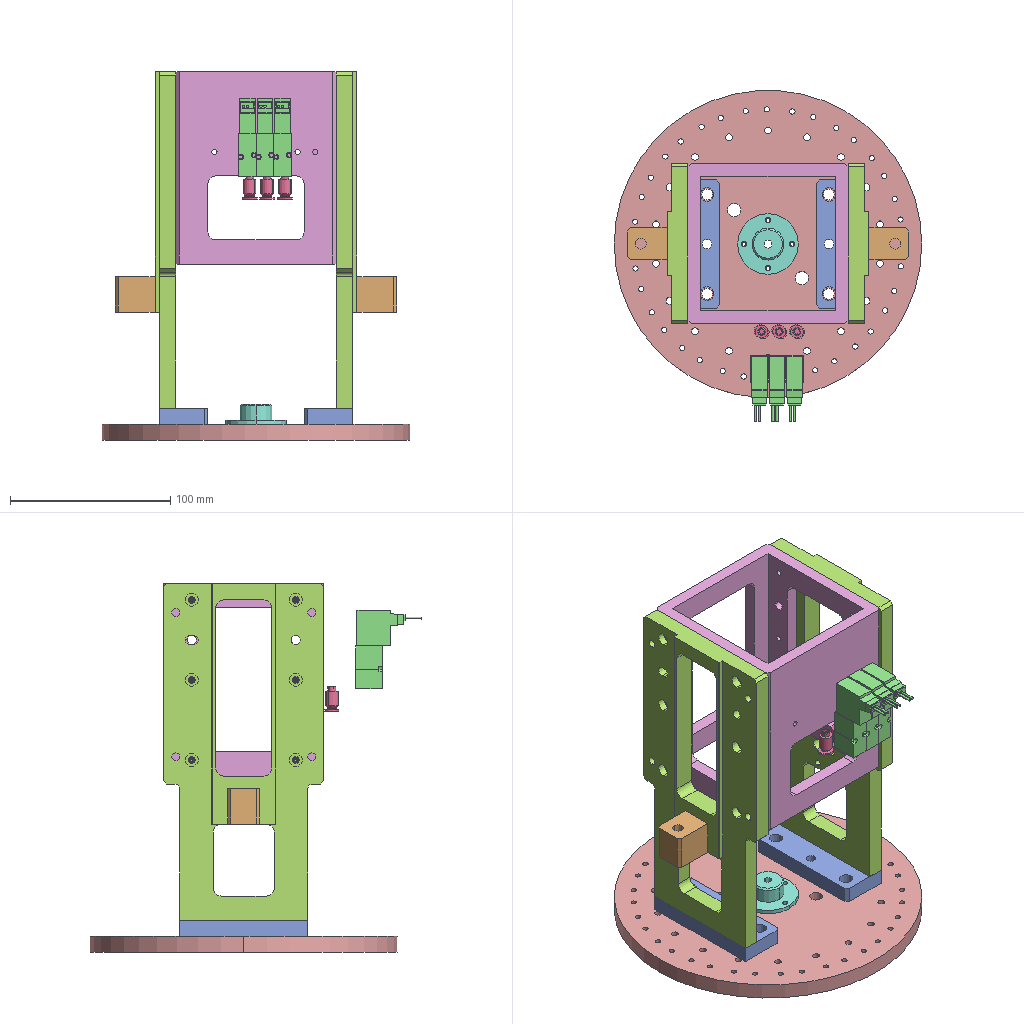Assembly | SolidWorks | 10 different items | 29 placed | box 192 x 207 x 230 mm
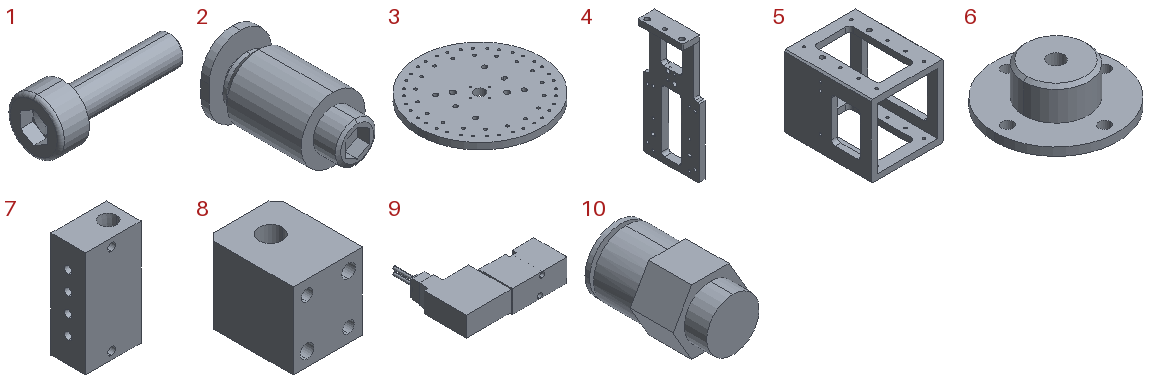Parts list (item | quantity | size | volume | features):
1 | x12 | 7.6 x 3 x 3 mm | 21.652 mm3 | features Fillet 2, RevCut 2, Boss 1, Chamfer 1, Cut 1, Extrusion 1, LPattern 1
2 | x4 | 8 x 15.6 x 9.8 mm | 520.13 mm3 | features BaseBody 1
3 | x1 | 192 x 192 x 10 mm | 278427 mm3 | features ICE 5, HoleWzd 3, 3DProfileFeature 2, CirPattern 2, Cut 2, Extrusion 1
4 | x2 | 33 x 100 x 220 mm | 162371 mm3 | features ICE 12, Chamfer 3, HoleWzd 3, Cut 2, Fillet 2, 3DProfileFeature 1, Extrusion 1
5 | x1 | 100 x 120 x 100 mm | 216402 mm3 | features ICE 5, HoleWzd 4, MirrorPattern 2, 3DProfileFeature 1, Chamfer 1, Cut 1, Extrusion 1
6 | x1 | 38 x 38 x 12.5 mm | 5119 mm3 | features ICE 2, Chamfer 1, Extrusion 1, HoleWzd 1
7 | x1 | 32 x 20 x 61 mm | 34864 mm3 | features HoleWzd 6, ICE 5, Extrusion 1, LPattern 1, RefAxis 1, RevCut 1
8 | x2 | 20 x 25 x 22 mm | 9700 mm3 | features HoleWzd 3, Chamfer 1, Extrusion 1
9 | x4 | 49 x 41 x 11 mm | 9805 mm3 | features BaseBody 1, ICE 1
10 | x1 | 13.856 x 21.6 x 12 mm | 1847 mm3 | features BaseBody 1
Mates (type | each side: item.copy, entity, surface, feature):
Coincident | 3.1 face plane Boss-Extrude1 | 4.1 face plane Boss-Extrude1
Coincident | 4.1 face plane Boss-Extrude1 | 5.1 face plane Boss-Extrude1
Coincident | 4.2 face plane Boss-Extrude1 | 5.1 face plane Boss-Extrude1
Concentric | 4.2 face cylinder Cut-Extrude7 | 5.1 face cylinder Mirror2
Concentric | 4.2 face cylinder Cut-Extrude8 | 5.1 face cylinder Mirror2
Concentric | 4.1 face cylinder Cut-Extrude7 | 1.1 face cylinder BaseBody
Coincident | 4.1 face plane Cut-Extrude8 | 1.1 face plane BaseHead
Concentric | 4.1 face cylinder Cut-Extrude7 | 1.2 face cylinder BaseBody
Coincident | 4.1 face plane Cut-Extrude8 | 1.2 face plane BaseHead
Concentric | 4.1 face cylinder Cut-Extrude7 | 1.3 face cylinder BaseBody
Coincident | 4.1 face plane Cut-Extrude8 | 1.3 face plane BaseHead
Concentric | 4.1 face cylinder Cut-Extrude7 | 1.4 face cylinder BaseBody
Coincident | 4.1 face plane Cut-Extrude8 | 1.4 face plane BaseHead
Concentric | 4.1 face cylinder Cut-Extrude7 | 1.5 face cylinder BaseBody
Coincident | 4.1 face plane Cut-Extrude8 | 1.5 face plane BaseHead
Concentric | 4.1 face cylinder Cut-Extrude7 | 1.6 face cylinder BaseBody
Coincident | 4.1 face plane Cut-Extrude8 | 1.6 face plane BaseHead
Concentric | 4.2 face cylinder Cut-Extrude7 | 1.7 face cylinder BaseBody
Coincident | 4.2 face plane Cut-Extrude8 | 1.7 face plane BaseHead
Concentric | 4.2 face cylinder Cut-Extrude8 | 1.8 face cylinder BaseBody
Coincident | 4.2 face plane Cut-Extrude8 | 1.8 face plane BaseHead
Concentric | 4.2 face cylinder Cut-Extrude8 | 1.9 face cylinder BaseBody
Coincident | 4.2 face plane Cut-Extrude8 | 1.9 face plane BaseHead
Concentric | 4.2 face cylinder Cut-Extrude8 | 1.10 face cylinder BaseBody
Coincident | 4.2 face plane Cut-Extrude8 | 1.10 face plane BaseHead
Concentric | 4.2 face cylinder Cut-Extrude7 | 1.11 face cylinder BaseBody
Coincident | 4.2 face plane Cut-Extrude8 | 1.11 face plane BaseHead
Concentric | 4.2 face cylinder Cut-Extrude7 | 1.12 face cylinder BaseBody
Coincident | 4.2 face plane Cut-Extrude8 | 1.12 face plane BaseHead
Concentric | 4.1 face cylinder Ø4.0 (4) Diameter Hole1 | 8.1 face cylinder Ø4.0 (4) Diameter Hole1
Coincident | 4.1 face plane Boss-Extrude3 | 8.1 face plane Boss-Extrude1 | 2 times
Concentric | 4.2 face cylinder Ø4.0 (4) Diameter Hole1 | 8.2 face cylinder Ø4.0 (4) Diameter Hole1
Coincident | 4.2 face plane Boss-Extrude3 | 8.2 face plane Boss-Extrude1 | 2 times
Concentric | 3.1 face cylinder M8 Tapped Hole2 | 4.2 face cylinder Cut-Extrude2 | 2 times
Concentric | 3.1 face cylinder M8 Tapped Hole2 | 4.1 face cylinder Cut-Extrude2 | 2 times
Concentric | 3.1 face cylinder Cut-Extrude1 | 6.1 face cylinder Boss-Extrude1
Coincident | 3.1 face plane Boss-Extrude1 | 6.1 face plane Boss-Extrude1
Concentric | 3.1 face cylinder M3 Tapped Hole1 | 6.1 face cylinder Cut-Extrude1
Concentric | 7.1 face cylinder M1.6 Tapped Hole1 | 9.1 face cylinder Input1
Parallel | 7.1 face plane Boss-Extrude1 | 9.1 face plane Input1
Coincident | 7.1 face plane Boss-Extrude1 | 9.1 face plane Input1
Concentric | 2.1 face cylinder Input1 | 7.1 face cylinder M5 Tapped Hole2
Coincident | 7.1 face plane Boss-Extrude1 | 2.1 face plane Input1
Concentric | 7.1 face cone 1/8 Rc Tapped Hole2 | 10.1 face cylinder Input1
Coincident | 7.1 face plane Boss-Extrude1 | 10.1 face plane Input1
Coincident | 5.1 face plane Boss-Extrude2 | 7.1 face plane Boss-Extrude1
Concentric | 5.1 face cylinder M4 Tapped Hole2 | 7.1 face cylinder Ø4.5 (4.5) Diameter Hole1 | 2 times